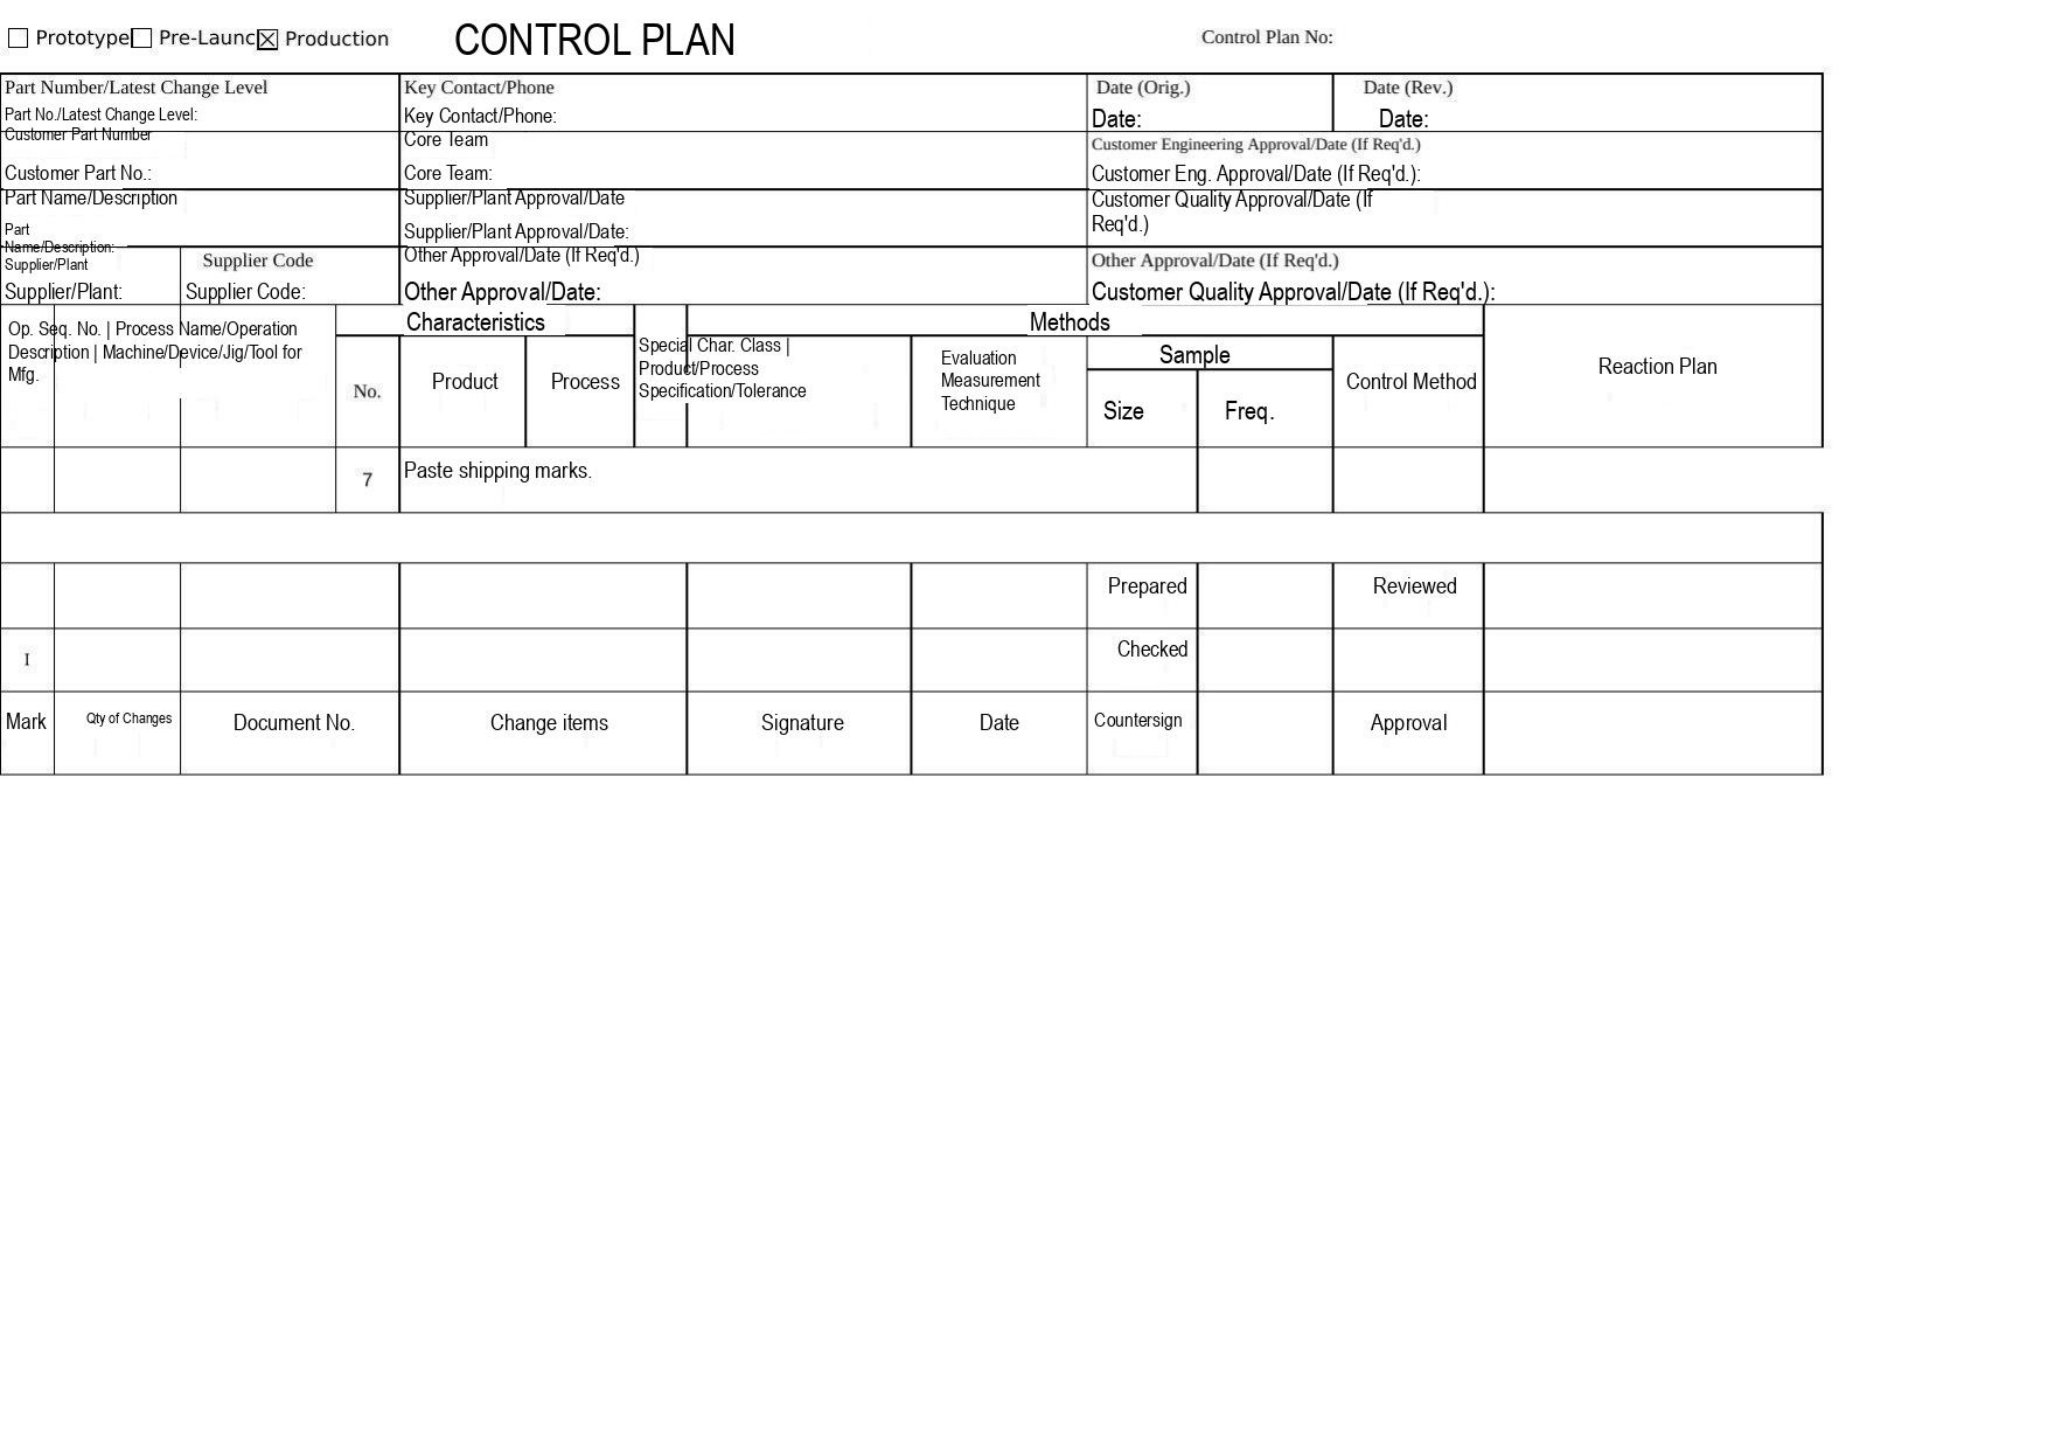☐ Prototype ☐ Pre-Launc ☒ Production CONTROL PLAN Control Plan No:

| Part Number/Latest Change Level<br>Part No./Latest Change Level: | Key Contact/Phone<br>Key Contact/Phone: | Date (Orig.)<br>Date: | Date (Rev.)<br>Date: |
|---|---|---|---|
| Customer Part Number<br>Customer Part No.: | Core Team<br>Core Team: | Customer Engineering Approval/Date (If Req'd.)<br>Customer Eng. Approval/Date (If Req'd.): | |
| Part Name/Description<br>Part Name/Description: | Supplier/Plant Approval/Date<br>Supplier/Plant Approval/Date: | Customer Quality Approval/Date (If Req'd.) | |
| Supplier/Plant<br>Supplier/Plant: · Supplier Code<br>Supplier Code: | Other Approval/Date (If Req'd.)<br>Other Approval/Date: | Other Approval/Date (If Req'd.)<br>Customer Quality Approval/Date (If Req'd.): | |

| Op. Seq. No. \| Process Name/Operation Description \| Machine/Device/Jig/Tool for Mfg. | | | Characteristics: No. | Characteristics: Product | Characteristics: Process | Special Char. Class \| Product/Process Specification/Tolerance | | Methods: Evaluation Measurement Technique | Methods: Sample Size | Methods: Sample Freq. | Methods: Control Method | Reaction Plan |
|---|---|---|---|---|---|---|---|---|---|---|---|---|
| | | | 7 | Paste shipping marks. | | | | | | | | |
| | | | | | | | | | | | | |
| | | | | | | | | | Prepared | | Reviewed | |
| I | | | | | | | | | Checked | | | |
| Mark | Qty of Changes | Document No. | | Change items | | | Signature | Date | Countersign | | Approval | |